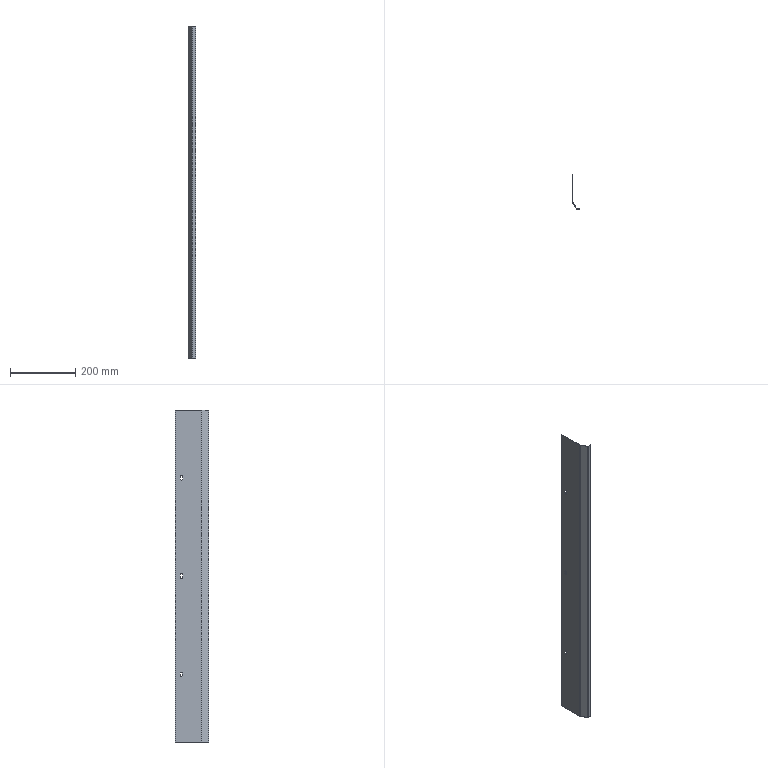Part | 1 solid | 37 faces | box 23.5 x 102.651 x 1015 mm | volume 117216 mm3 | plane 24 | cylinder 13 | commonest cylinder face diameters 7 x6 6 x3 1 x2 3 x2
STEP:
#1=CARTESIAN_POINT('',(0.,-16.,-296.5));
#2=VERTEX_POINT('',#1);
#3=CARTESIAN_POINT('',(0.,-19.,-293.5));
#4=VERTEX_POINT('',#3);
#5=CARTESIAN_POINT('',(0.,-19.,-296.5));
#6=DIRECTION('',(1.,0.,0.));
#7=DIRECTION('',(0.,1.,0.));
#8=AXIS2_PLACEMENT_3D('',#5,#6,#7);
#9=CIRCLE('',#8,3.);
#10=EDGE_CURVE('',#2,#4,#9,.T.);
#11=ORIENTED_EDGE('',*,*,#10,.T.);
#12=CARTESIAN_POINT('',(-1.,-19.,-293.5));
#13=VERTEX_POINT('',#12);
#14=CARTESIAN_POINT('',(9.,-19.,-293.5));
#15=DIRECTION('',(-1.,0.,0.));
#16=VECTOR('',#15,1000.);
#17=LINE('',#14,#16);
#18=EDGE_CURVE('',#4,#13,#17,.T.);
#19=ORIENTED_EDGE('',*,*,#18,.T.);
#20=CARTESIAN_POINT('',(-1.,-16.,-296.5));
#21=VERTEX_POINT('',#20);
#22=CARTESIAN_POINT('',(-1.,-19.,-296.5));
#23=DIRECTION('',(-1.,0.,0.));
#24=DIRECTION('',(0.,0.,1.));
#25=AXIS2_PLACEMENT_3D('',#22,#23,#24);
#26=CIRCLE('',#25,3.);
#27=EDGE_CURVE('',#13,#21,#26,.T.);
#28=ORIENTED_EDGE('',*,*,#27,.T.);
#29=CARTESIAN_POINT('',(9.,-16.,-296.5));
#30=DIRECTION('',(-1.,0.,0.));
#31=VECTOR('',#30,1000.);
#32=LINE('',#29,#31);
#33=EDGE_CURVE('',#2,#21,#32,.T.);
#34=ORIENTED_EDGE('',*,*,#33,.F.);
#35=EDGE_LOOP('',(#11,#19,#28,#34));
#36=FACE_OUTER_BOUND('',#35,.T.);
#37=CARTESIAN_POINT('',(9.,-19.,-296.5));
#38=DIRECTION('',(-1.,0.,0.));
#39=DIRECTION('',(0.,0.,1.));
#40=AXIS2_PLACEMENT_3D('',#37,#38,#39);
#41=CYLINDRICAL_SURFACE('',#40,3.);
#42=ADVANCED_FACE('',(#36),#41,.F.);
#43=CARTESIAN_POINT('',(0.,-15.5,303.5));
#44=VERTEX_POINT('',#43);
#45=CARTESIAN_POINT('',(0.,-19.,307.));
#46=VERTEX_POINT('',#45);
#47=CARTESIAN_POINT('',(0.,-19.,303.5));
#48=DIRECTION('',(1.,0.,0.));
#49=DIRECTION('',(0.,1.,0.));
#50=AXIS2_PLACEMENT_3D('',#47,#48,#49);
#51=CIRCLE('',#50,3.5);
#52=EDGE_CURVE('',#44,#46,#51,.T.);
#53=ORIENTED_EDGE('',*,*,#52,.T.);
#54=CARTESIAN_POINT('',(-1.,-19.,307.));
#55=VERTEX_POINT('',#54);
#56=CARTESIAN_POINT('',(9.,-19.,307.));
#57=DIRECTION('',(-1.,0.,0.));
#58=VECTOR('',#57,1000.);
#59=LINE('',#56,#58);
#60=EDGE_CURVE('',#46,#55,#59,.T.);
#61=ORIENTED_EDGE('',*,*,#60,.T.);
#62=CARTESIAN_POINT('',(-1.,-15.5,303.5));
#63=VERTEX_POINT('',#62);
#64=CARTESIAN_POINT('',(-1.,-19.,303.5));
#65=DIRECTION('',(-1.,0.,0.));
#66=DIRECTION('',(0.,0.,1.));
#67=AXIS2_PLACEMENT_3D('',#64,#65,#66);
#68=CIRCLE('',#67,3.5);
#69=EDGE_CURVE('',#55,#63,#68,.T.);
#70=ORIENTED_EDGE('',*,*,#69,.T.);
#71=CARTESIAN_POINT('',(9.,-15.5,303.5));
#72=DIRECTION('',(-1.,0.,0.));
#73=VECTOR('',#72,1000.);
#74=LINE('',#71,#73);
#75=EDGE_CURVE('',#44,#63,#74,.T.);
#76=ORIENTED_EDGE('',*,*,#75,.F.);
#77=EDGE_LOOP('',(#53,#61,#70,#76));
#78=FACE_OUTER_BOUND('',#77,.T.);
#79=CARTESIAN_POINT('',(9.,-19.,303.5));
#80=DIRECTION('',(-1.,0.,0.));
#81=DIRECTION('',(0.,0.,1.));
#82=AXIS2_PLACEMENT_3D('',#79,#80,#81);
#83=CYLINDRICAL_SURFACE('',#82,3.5);
#84=ADVANCED_FACE('',(#78),#83,.F.);
#85=CARTESIAN_POINT('',(0.,-15.5,3.5));
#86=VERTEX_POINT('',#85);
#87=CARTESIAN_POINT('',(0.,-19.,7.));
#88=VERTEX_POINT('',#87);
#89=CARTESIAN_POINT('',(0.,-19.,3.5));
#90=DIRECTION('',(1.,0.,0.));
#91=DIRECTION('',(0.,1.,0.));
#92=AXIS2_PLACEMENT_3D('',#89,#90,#91);
#93=CIRCLE('',#92,3.5);
#94=EDGE_CURVE('',#86,#88,#93,.T.);
#95=ORIENTED_EDGE('',*,*,#94,.T.);
#96=CARTESIAN_POINT('',(-1.,-19.,7.));
#97=VERTEX_POINT('',#96);
#98=CARTESIAN_POINT('',(9.,-19.,7.));
#99=DIRECTION('',(-1.,0.,0.));
#100=VECTOR('',#99,1000.);
#101=LINE('',#98,#100);
#102=EDGE_CURVE('',#88,#97,#101,.T.);
#103=ORIENTED_EDGE('',*,*,#102,.T.);
#104=CARTESIAN_POINT('',(-1.,-15.5,3.5));
#105=VERTEX_POINT('',#104);
#106=CARTESIAN_POINT('',(-1.,-19.,3.5));
#107=DIRECTION('',(-1.,0.,0.));
#108=DIRECTION('',(0.,0.,1.));
#109=AXIS2_PLACEMENT_3D('',#106,#107,#108);
#110=CIRCLE('',#109,3.5);
#111=EDGE_CURVE('',#97,#105,#110,.T.);
#112=ORIENTED_EDGE('',*,*,#111,.T.);
#113=CARTESIAN_POINT('',(9.,-15.5,3.5));
#114=DIRECTION('',(-1.,0.,0.));
#115=VECTOR('',#114,1000.);
#116=LINE('',#113,#115);
#117=EDGE_CURVE('',#86,#105,#116,.T.);
#118=ORIENTED_EDGE('',*,*,#117,.F.);
#119=EDGE_LOOP('',(#95,#103,#112,#118));
#120=FACE_OUTER_BOUND('',#119,.T.);
#121=CARTESIAN_POINT('',(9.,-19.,3.5));
#122=DIRECTION('',(-1.,0.,0.));
#123=DIRECTION('',(0.,0.,1.));
#124=AXIS2_PLACEMENT_3D('',#121,#122,#123);
#125=CYLINDRICAL_SURFACE('',#124,3.5);
#126=ADVANCED_FACE('',(#120),#125,.F.);
#127=CARTESIAN_POINT('',(0.06699,-80.116,507.5));
#128=VERTEX_POINT('',#127);
#129=CARTESIAN_POINT('',(-0.799,-80.616,507.5));
#130=VERTEX_POINT('',#129);
#131=CARTESIAN_POINT('',(0.06699,-80.116,507.5));
#132=DIRECTION('',(-0.866,-0.5,0.));
#133=VECTOR('',#132,1000.);
#134=LINE('',#131,#133);
#135=EDGE_CURVE('',#128,#130,#134,.T.);
#136=ORIENTED_EDGE('',*,*,#135,.F.);
#137=CARTESIAN_POINT('',(0.,-79.866,507.5));
#138=VERTEX_POINT('',#137);
#139=CARTESIAN_POINT('',(0.5,-79.866,507.5));
#140=DIRECTION('',(0.,0.,1.));
#141=DIRECTION('',(-1.,0.,0.));
#142=AXIS2_PLACEMENT_3D('',#139,#140,#141);
#143=CIRCLE('',#142,0.5);
#144=EDGE_CURVE('',#138,#128,#143,.T.);
#145=ORIENTED_EDGE('',*,*,#144,.F.);
#146=CARTESIAN_POINT('',(-1.,-79.866,507.5));
#147=VERTEX_POINT('',#146);
#148=CARTESIAN_POINT('',(-1.,-79.866,507.5));
#149=DIRECTION('',(1.,0.,0.));
#150=VECTOR('',#149,1000.);
#151=LINE('',#148,#150);
#152=EDGE_CURVE('',#147,#138,#151,.T.);
#153=ORIENTED_EDGE('',*,*,#152,.F.);
#154=CARTESIAN_POINT('',(0.5,-79.866,507.5));
#155=DIRECTION('',(0.,0.,1.));
#156=DIRECTION('',(1.,0.,0.));
#157=AXIS2_PLACEMENT_3D('',#154,#155,#156);
#158=CIRCLE('',#157,1.5);
#159=EDGE_CURVE('',#147,#130,#158,.T.);
#160=ORIENTED_EDGE('',*,*,#159,.T.);
#161=EDGE_LOOP('',(#136,#145,#153,#160));
#162=FACE_OUTER_BOUND('',#161,.T.);
#163=CARTESIAN_POINT('',(0.06699,-80.116,507.5));
#164=DIRECTION('',(0.,0.,1.));
#165=DIRECTION('',(1.,0.,0.));
#166=AXIS2_PLACEMENT_3D('',#163,#164,#165);
#167=PLANE('',#166);
#168=ADVANCED_FACE('',(#162),#167,.T.);
#169=CARTESIAN_POINT('',(12.356,-101.401,507.5));
#170=VERTEX_POINT('',#169);
#171=CARTESIAN_POINT('',(0.,-80.,507.5));
#172=DIRECTION('',(0.5,-0.866,0.));
#173=VECTOR('',#172,1000.);
#174=LINE('',#171,#173);
#175=EDGE_CURVE('',#128,#170,#174,.T.);
#176=ORIENTED_EDGE('',*,*,#175,.F.);
#177=ORIENTED_EDGE('',*,*,#135,.T.);
#178=CARTESIAN_POINT('',(11.49,-101.901,507.5));
#179=VERTEX_POINT('',#178);
#180=CARTESIAN_POINT('',(-0.866,-80.5,507.5));
#181=DIRECTION('',(0.5,-0.866,0.));
#182=VECTOR('',#181,1000.);
#183=LINE('',#180,#182);
#184=EDGE_CURVE('',#130,#179,#183,.T.);
#185=ORIENTED_EDGE('',*,*,#184,.T.);
#186=CARTESIAN_POINT('',(11.49,-101.901,507.5));
#187=DIRECTION('',(0.866,0.5,0.));
#188=VECTOR('',#187,1000.);
#189=LINE('',#186,#188);
#190=EDGE_CURVE('',#179,#170,#189,.T.);
#191=ORIENTED_EDGE('',*,*,#190,.T.);
#192=EDGE_LOOP('',(#176,#177,#185,#191));
#193=FACE_OUTER_BOUND('',#192,.T.);
#194=CARTESIAN_POINT('',(-1.,-79.866,507.5));
#195=DIRECTION('',(0.,0.,1.));
#196=DIRECTION('',(1.,0.,0.));
#197=AXIS2_PLACEMENT_3D('',#194,#195,#196);
#198=PLANE('',#197);
#199=ADVANCED_FACE('',(#193),#198,.T.);
#200=CARTESIAN_POINT('',(0.,-79.866,-507.5));
#201=VERTEX_POINT('',#200);
#202=CARTESIAN_POINT('',(-1.,-79.866,-507.5));
#203=VERTEX_POINT('',#202);
#204=CARTESIAN_POINT('',(0.,-79.866,-507.5));
#205=DIRECTION('',(-1.,0.,0.));
#206=VECTOR('',#205,1000.);
#207=LINE('',#204,#206);
#208=EDGE_CURVE('',#201,#203,#207,.T.);
#209=ORIENTED_EDGE('',*,*,#208,.F.);
#210=CARTESIAN_POINT('',(0.06699,-80.116,-507.5));
#211=VERTEX_POINT('',#210);
#212=CARTESIAN_POINT('',(0.5,-79.866,-507.5));
#213=DIRECTION('',(0.,0.,1.));
#214=DIRECTION('',(-1.,0.,0.));
#215=AXIS2_PLACEMENT_3D('',#212,#213,#214);
#216=CIRCLE('',#215,0.5);
#217=EDGE_CURVE('',#201,#211,#216,.T.);
#218=ORIENTED_EDGE('',*,*,#217,.T.);
#219=CARTESIAN_POINT('',(-0.799,-80.616,-507.5));
#220=VERTEX_POINT('',#219);
#221=CARTESIAN_POINT('',(-0.799,-80.616,-507.5));
#222=DIRECTION('',(0.866,0.5,0.));
#223=VECTOR('',#222,1000.);
#224=LINE('',#221,#223);
#225=EDGE_CURVE('',#220,#211,#224,.T.);
#226=ORIENTED_EDGE('',*,*,#225,.F.);
#227=CARTESIAN_POINT('',(0.5,-79.866,-507.5));
#228=DIRECTION('',(0.,0.,1.));
#229=DIRECTION('',(1.,0.,0.));
#230=AXIS2_PLACEMENT_3D('',#227,#228,#229);
#231=CIRCLE('',#230,1.5);
#232=EDGE_CURVE('',#203,#220,#231,.T.);
#233=ORIENTED_EDGE('',*,*,#232,.F.);
#234=EDGE_LOOP('',(#209,#218,#226,#233));
#235=FACE_OUTER_BOUND('',#234,.T.);
#236=CARTESIAN_POINT('',(0.,-79.866,-507.5));
#237=DIRECTION('',(0.,0.,-1.));
#238=DIRECTION('',(-1.,0.,0.));
#239=AXIS2_PLACEMENT_3D('',#236,#237,#238);
#240=PLANE('',#239);
#241=ADVANCED_FACE('',(#235),#240,.T.);
#242=CARTESIAN_POINT('',(0.,0.,-507.5));
#243=VERTEX_POINT('',#242);
#244=CARTESIAN_POINT('',(0.,0.,-507.5));
#245=DIRECTION('',(0.,-1.,0.));
#246=VECTOR('',#245,1000.);
#247=LINE('',#244,#246);
#248=EDGE_CURVE('',#243,#201,#247,.T.);
#249=ORIENTED_EDGE('',*,*,#248,.T.);
#250=ORIENTED_EDGE('',*,*,#208,.T.);
#251=CARTESIAN_POINT('',(-1.,0.,-507.5));
#252=VERTEX_POINT('',#251);
#253=CARTESIAN_POINT('',(-1.,0.,-507.5));
#254=DIRECTION('',(0.,-1.,0.));
#255=VECTOR('',#254,1000.);
#256=LINE('',#253,#255);
#257=EDGE_CURVE('',#252,#203,#256,.T.);
#258=ORIENTED_EDGE('',*,*,#257,.F.);
#259=CARTESIAN_POINT('',(-1.,0.,-507.5));
#260=DIRECTION('',(1.,0.,0.));
#261=VECTOR('',#260,1000.);
#262=LINE('',#259,#261);
#263=EDGE_CURVE('',#252,#243,#262,.T.);
#264=ORIENTED_EDGE('',*,*,#263,.T.);
#265=EDGE_LOOP('',(#249,#250,#258,#264));
#266=FACE_OUTER_BOUND('',#265,.T.);
#267=CARTESIAN_POINT('',(-0.799,-80.616,-507.5));
#268=DIRECTION('',(0.,0.,-1.));
#269=DIRECTION('',(-1.,0.,0.));
#270=AXIS2_PLACEMENT_3D('',#267,#268,#269);
#271=PLANE('',#270);
#272=ADVANCED_FACE('',(#266),#271,.T.);
#273=CARTESIAN_POINT('',(12.789,-101.651,507.5));
#274=VERTEX_POINT('',#273);
#275=CARTESIAN_POINT('',(12.789,-102.651,507.5));
#276=VERTEX_POINT('',#275);
#277=CARTESIAN_POINT('',(12.789,-101.651,507.5));
#278=DIRECTION('',(0.,-1.,0.));
#279=VECTOR('',#278,1000.);
#280=LINE('',#277,#279);
#281=EDGE_CURVE('',#274,#276,#280,.T.);
#282=ORIENTED_EDGE('',*,*,#281,.F.);
#283=CARTESIAN_POINT('',(12.789,-101.151,507.5));
#284=DIRECTION('',(0.,0.,1.));
#285=DIRECTION('',(-1.,0.,0.));
#286=AXIS2_PLACEMENT_3D('',#283,#284,#285);
#287=CIRCLE('',#286,0.5);
#288=EDGE_CURVE('',#170,#274,#287,.T.);
#289=ORIENTED_EDGE('',*,*,#288,.F.);
#290=ORIENTED_EDGE('',*,*,#190,.F.);
#291=CARTESIAN_POINT('',(12.789,-101.151,507.5));
#292=DIRECTION('',(0.,0.,1.));
#293=DIRECTION('',(1.,0.,0.));
#294=AXIS2_PLACEMENT_3D('',#291,#292,#293);
#295=CIRCLE('',#294,1.5);
#296=EDGE_CURVE('',#179,#276,#295,.T.);
#297=ORIENTED_EDGE('',*,*,#296,.T.);
#298=EDGE_LOOP('',(#282,#289,#290,#297));
#299=FACE_OUTER_BOUND('',#298,.T.);
#300=CARTESIAN_POINT('',(12.789,-101.651,507.5));
#301=DIRECTION('',(0.,0.,1.));
#302=DIRECTION('',(1.,0.,0.));
#303=AXIS2_PLACEMENT_3D('',#300,#301,#302);
#304=PLANE('',#303);
#305=ADVANCED_FACE('',(#299),#304,.T.);
#306=CARTESIAN_POINT('',(22.5,-101.651,507.5));
#307=VERTEX_POINT('',#306);
#308=CARTESIAN_POINT('',(12.5,-101.651,507.5));
#309=DIRECTION('',(1.,0.,0.));
#310=VECTOR('',#309,1000.);
#311=LINE('',#308,#310);
#312=EDGE_CURVE('',#274,#307,#311,.T.);
#313=ORIENTED_EDGE('',*,*,#312,.F.);
#314=ORIENTED_EDGE('',*,*,#281,.T.);
#315=CARTESIAN_POINT('',(22.5,-102.651,507.5));
#316=VERTEX_POINT('',#315);
#317=CARTESIAN_POINT('',(12.5,-102.651,507.5));
#318=DIRECTION('',(1.,0.,0.));
#319=VECTOR('',#318,1000.);
#320=LINE('',#317,#319);
#321=EDGE_CURVE('',#276,#316,#320,.T.);
#322=ORIENTED_EDGE('',*,*,#321,.T.);
#323=CARTESIAN_POINT('',(22.5,-101.651,507.5));
#324=DIRECTION('',(0.,-1.,0.));
#325=VECTOR('',#324,1000.);
#326=LINE('',#323,#325);
#327=EDGE_CURVE('',#307,#316,#326,.T.);
#328=ORIENTED_EDGE('',*,*,#327,.F.);
#329=EDGE_LOOP('',(#313,#314,#322,#328));
#330=FACE_OUTER_BOUND('',#329,.T.);
#331=CARTESIAN_POINT('',(11.49,-101.901,507.5));
#332=DIRECTION('',(0.,0.,1.));
#333=DIRECTION('',(1.,0.,0.));
#334=AXIS2_PLACEMENT_3D('',#331,#332,#333);
#335=PLANE('',#334);
#336=ADVANCED_FACE('',(#330),#335,.T.);
#337=CARTESIAN_POINT('',(12.356,-101.401,-507.5));
#338=VERTEX_POINT('',#337);
#339=CARTESIAN_POINT('',(11.49,-101.901,-507.5));
#340=VERTEX_POINT('',#339);
#341=CARTESIAN_POINT('',(12.356,-101.401,-507.5));
#342=DIRECTION('',(-0.866,-0.5,0.));
#343=VECTOR('',#342,1000.);
#344=LINE('',#341,#343);
#345=EDGE_CURVE('',#338,#340,#344,.T.);
#346=ORIENTED_EDGE('',*,*,#345,.F.);
#347=CARTESIAN_POINT('',(12.789,-101.651,-507.5));
#348=VERTEX_POINT('',#347);
#349=CARTESIAN_POINT('',(12.789,-101.151,-507.5));
#350=DIRECTION('',(0.,0.,1.));
#351=DIRECTION('',(-1.,0.,0.));
#352=AXIS2_PLACEMENT_3D('',#349,#350,#351);
#353=CIRCLE('',#352,0.5);
#354=EDGE_CURVE('',#338,#348,#353,.T.);
#355=ORIENTED_EDGE('',*,*,#354,.T.);
#356=CARTESIAN_POINT('',(12.789,-102.651,-507.5));
#357=VERTEX_POINT('',#356);
#358=CARTESIAN_POINT('',(12.789,-102.651,-507.5));
#359=DIRECTION('',(0.,1.,0.));
#360=VECTOR('',#359,1000.);
#361=LINE('',#358,#360);
#362=EDGE_CURVE('',#357,#348,#361,.T.);
#363=ORIENTED_EDGE('',*,*,#362,.F.);
#364=CARTESIAN_POINT('',(12.789,-101.151,-507.5));
#365=DIRECTION('',(0.,0.,1.));
#366=DIRECTION('',(1.,0.,0.));
#367=AXIS2_PLACEMENT_3D('',#364,#365,#366);
#368=CIRCLE('',#367,1.5);
#369=EDGE_CURVE('',#340,#357,#368,.T.);
#370=ORIENTED_EDGE('',*,*,#369,.F.);
#371=EDGE_LOOP('',(#346,#355,#363,#370));
#372=FACE_OUTER_BOUND('',#371,.T.);
#373=CARTESIAN_POINT('',(12.356,-101.401,-507.5));
#374=DIRECTION('',(0.,0.,-1.));
#375=DIRECTION('',(-1.,0.,0.));
#376=AXIS2_PLACEMENT_3D('',#373,#374,#375);
#377=PLANE('',#376);
#378=ADVANCED_FACE('',(#372),#377,.T.);
#379=CARTESIAN_POINT('',(0.,-80.,-507.5));
#380=DIRECTION('',(0.5,-0.866,0.));
#381=VECTOR('',#380,1000.);
#382=LINE('',#379,#381);
#383=EDGE_CURVE('',#211,#338,#382,.T.);
#384=ORIENTED_EDGE('',*,*,#383,.T.);
#385=ORIENTED_EDGE('',*,*,#345,.T.);
#386=CARTESIAN_POINT('',(-0.866,-80.5,-507.5));
#387=DIRECTION('',(0.5,-0.866,0.));
#388=VECTOR('',#387,1000.);
#389=LINE('',#386,#388);
#390=EDGE_CURVE('',#220,#340,#389,.T.);
#391=ORIENTED_EDGE('',*,*,#390,.F.);
#392=ORIENTED_EDGE('',*,*,#225,.T.);
#393=EDGE_LOOP('',(#384,#385,#391,#392));
#394=FACE_OUTER_BOUND('',#393,.T.);
#395=CARTESIAN_POINT('',(12.789,-102.651,-507.5));
#396=DIRECTION('',(0.,0.,-1.));
#397=DIRECTION('',(-1.,0.,0.));
#398=AXIS2_PLACEMENT_3D('',#395,#396,#397);
#399=PLANE('',#398);
#400=ADVANCED_FACE('',(#394),#399,.T.);
#401=CARTESIAN_POINT('',(22.5,-102.651,-507.5));
#402=VERTEX_POINT('',#401);
#403=CARTESIAN_POINT('',(12.5,-102.651,-507.5));
#404=DIRECTION('',(1.,0.,0.));
#405=VECTOR('',#404,1000.);
#406=LINE('',#403,#405);
#407=EDGE_CURVE('',#357,#402,#406,.T.);
#408=ORIENTED_EDGE('',*,*,#407,.T.);
#409=CARTESIAN_POINT('',(22.5,-102.651,507.5));
#410=DIRECTION('',(0.,0.,-1.));
#411=VECTOR('',#410,1000.);
#412=LINE('',#409,#411);
#413=EDGE_CURVE('',#316,#402,#412,.T.);
#414=ORIENTED_EDGE('',*,*,#413,.F.);
#415=ORIENTED_EDGE('',*,*,#321,.F.);
#416=CARTESIAN_POINT('',(12.789,-102.651,507.5));
#417=DIRECTION('',(0.,0.,-1.));
#418=VECTOR('',#417,1000.);
#419=LINE('',#416,#418);
#420=EDGE_CURVE('',#276,#357,#419,.T.);
#421=ORIENTED_EDGE('',*,*,#420,.T.);
#422=EDGE_LOOP('',(#408,#414,#415,#421));
#423=FACE_OUTER_BOUND('',#422,.T.);
#424=CARTESIAN_POINT('',(12.5,-102.651,507.5));
#425=DIRECTION('',(0.,1.,0.));
#426=DIRECTION('',(0.,0.,1.));
#427=AXIS2_PLACEMENT_3D('',#424,#425,#426);
#428=PLANE('',#427);
#429=ADVANCED_FACE('',(#423),#428,.F.);
#430=CARTESIAN_POINT('',(22.5,-101.651,-507.5));
#431=VERTEX_POINT('',#430);
#432=CARTESIAN_POINT('',(22.5,-101.651,-507.5));
#433=DIRECTION('',(0.,-1.,0.));
#434=VECTOR('',#433,1000.);
#435=LINE('',#432,#434);
#436=EDGE_CURVE('',#431,#402,#435,.T.);
#437=ORIENTED_EDGE('',*,*,#436,.F.);
#438=CARTESIAN_POINT('',(22.5,-101.651,507.5));
#439=DIRECTION('',(0.,0.,-1.));
#440=VECTOR('',#439,1000.);
#441=LINE('',#438,#440);
#442=EDGE_CURVE('',#307,#431,#441,.T.);
#443=ORIENTED_EDGE('',*,*,#442,.F.);
#444=ORIENTED_EDGE('',*,*,#327,.T.);
#445=ORIENTED_EDGE('',*,*,#413,.T.);
#446=EDGE_LOOP('',(#437,#443,#444,#445));
#447=FACE_OUTER_BOUND('',#446,.T.);
#448=CARTESIAN_POINT('',(22.5,-101.651,507.5));
#449=DIRECTION('',(1.,0.,0.));
#450=DIRECTION('',(0.,0.,-1.));
#451=AXIS2_PLACEMENT_3D('',#448,#449,#450);
#452=PLANE('',#451);
#453=ADVANCED_FACE('',(#447),#452,.T.);
#454=CARTESIAN_POINT('',(12.5,-101.651,-507.5));
#455=DIRECTION('',(1.,0.,0.));
#456=VECTOR('',#455,1000.);
#457=LINE('',#454,#456);
#458=EDGE_CURVE('',#348,#431,#457,.T.);
#459=ORIENTED_EDGE('',*,*,#458,.F.);
#460=CARTESIAN_POINT('',(12.789,-101.651,507.5));
#461=DIRECTION('',(0.,0.,-1.));
#462=VECTOR('',#461,1000.);
#463=LINE('',#460,#462);
#464=EDGE_CURVE('',#274,#348,#463,.T.);
#465=ORIENTED_EDGE('',*,*,#464,.F.);
#466=ORIENTED_EDGE('',*,*,#312,.T.);
#467=ORIENTED_EDGE('',*,*,#442,.T.);
#468=EDGE_LOOP('',(#459,#465,#466,#467));
#469=FACE_OUTER_BOUND('',#468,.T.);
#470=CARTESIAN_POINT('',(12.5,-101.651,507.5));
#471=DIRECTION('',(0.,1.,0.));
#472=DIRECTION('',(0.,0.,1.));
#473=AXIS2_PLACEMENT_3D('',#470,#471,#472);
#474=PLANE('',#473);
#475=ADVANCED_FACE('',(#469),#474,.T.);
#476=ORIENTED_EDGE('',*,*,#354,.F.);
#477=CARTESIAN_POINT('',(12.356,-101.401,507.5));
#478=DIRECTION('',(0.,0.,-1.));
#479=VECTOR('',#478,1000.);
#480=LINE('',#477,#479);
#481=EDGE_CURVE('',#170,#338,#480,.T.);
#482=ORIENTED_EDGE('',*,*,#481,.F.);
#483=ORIENTED_EDGE('',*,*,#288,.T.);
#484=ORIENTED_EDGE('',*,*,#464,.T.);
#485=EDGE_LOOP('',(#476,#482,#483,#484));
#486=FACE_OUTER_BOUND('',#485,.T.);
#487=CARTESIAN_POINT('',(12.789,-101.151,507.5));
#488=DIRECTION('',(0.,0.,-1.));
#489=DIRECTION('',(-1.,0.,0.));
#490=AXIS2_PLACEMENT_3D('',#487,#488,#489);
#491=CYLINDRICAL_SURFACE('',#490,0.5);
#492=ADVANCED_FACE('',(#486),#491,.F.);
#493=ORIENTED_EDGE('',*,*,#383,.F.);
#494=CARTESIAN_POINT('',(0.06699,-80.116,507.5));
#495=DIRECTION('',(0.,0.,-1.));
#496=VECTOR('',#495,1000.);
#497=LINE('',#494,#496);
#498=EDGE_CURVE('',#128,#211,#497,.T.);
#499=ORIENTED_EDGE('',*,*,#498,.F.);
#500=ORIENTED_EDGE('',*,*,#175,.T.);
#501=ORIENTED_EDGE('',*,*,#481,.T.);
#502=EDGE_LOOP('',(#493,#499,#500,#501));
#503=FACE_OUTER_BOUND('',#502,.T.);
#504=CARTESIAN_POINT('',(0.,-80.,507.5));
#505=DIRECTION('',(0.866,0.5,0.));
#506=DIRECTION('',(-0.5,0.866,0.));
#507=AXIS2_PLACEMENT_3D('',#504,#505,#506);
#508=PLANE('',#507);
#509=ADVANCED_FACE('',(#503),#508,.T.);
#510=ORIENTED_EDGE('',*,*,#217,.F.);
#511=CARTESIAN_POINT('',(0.,-79.866,507.5));
#512=DIRECTION('',(0.,0.,-1.));
#513=VECTOR('',#512,1000.);
#514=LINE('',#511,#513);
#515=EDGE_CURVE('',#138,#201,#514,.T.);
#516=ORIENTED_EDGE('',*,*,#515,.F.);
#517=ORIENTED_EDGE('',*,*,#144,.T.);
#518=ORIENTED_EDGE('',*,*,#498,.T.);
#519=EDGE_LOOP('',(#510,#516,#517,#518));
#520=FACE_OUTER_BOUND('',#519,.T.);
#521=CARTESIAN_POINT('',(0.5,-79.866,507.5));
#522=DIRECTION('',(0.,0.,-1.));
#523=DIRECTION('',(-1.,0.,0.));
#524=AXIS2_PLACEMENT_3D('',#521,#522,#523);
#525=CYLINDRICAL_SURFACE('',#524,0.5);
#526=ADVANCED_FACE('',(#520),#525,.F.);
#527=CARTESIAN_POINT('',(0.,-22.,-303.5));
#528=VERTEX_POINT('',#527);
#529=CARTESIAN_POINT('',(0.,-16.,-303.5));
#530=VERTEX_POINT('',#529);
#531=CARTESIAN_POINT('',(0.,-19.,-303.5));
#532=DIRECTION('',(1.,0.,0.));
#533=DIRECTION('',(0.,1.,0.));
#534=AXIS2_PLACEMENT_3D('',#531,#532,#533);
#535=CIRCLE('',#534,3.);
#536=EDGE_CURVE('',#528,#530,#535,.T.);
#537=ORIENTED_EDGE('',*,*,#536,.F.);
#538=CARTESIAN_POINT('',(0.,-22.,-296.5));
#539=VERTEX_POINT('',#538);
#540=CARTESIAN_POINT('',(0.,-22.,507.5));
#541=DIRECTION('',(0.,0.,-1.));
#542=VECTOR('',#541,1000.);
#543=LINE('',#540,#542);
#544=EDGE_CURVE('',#539,#528,#543,.T.);
#545=ORIENTED_EDGE('',*,*,#544,.F.);
#546=CARTESIAN_POINT('',(0.,-19.,-296.5));
#547=DIRECTION('',(1.,0.,0.));
#548=DIRECTION('',(0.,1.,0.));
#549=AXIS2_PLACEMENT_3D('',#546,#547,#548);
#550=CIRCLE('',#549,3.);
#551=EDGE_CURVE('',#4,#539,#550,.T.);
#552=ORIENTED_EDGE('',*,*,#551,.F.);
#553=ORIENTED_EDGE('',*,*,#10,.F.);
#554=CARTESIAN_POINT('',(0.,-16.,507.5));
#555=DIRECTION('',(0.,0.,1.));
#556=VECTOR('',#555,1000.);
#557=LINE('',#554,#556);
#558=EDGE_CURVE('',#530,#2,#557,.T.);
#559=ORIENTED_EDGE('',*,*,#558,.F.);
#560=EDGE_LOOP('',(#537,#545,#552,#553,#559));
#561=FACE_BOUND('',#560,.T.);
#562=CARTESIAN_POINT('',(0.,-22.5,296.5));
#563=VERTEX_POINT('',#562);
#564=CARTESIAN_POINT('',(0.,-15.5,296.5));
#565=VERTEX_POINT('',#564);
#566=CARTESIAN_POINT('',(0.,-19.,296.5));
#567=DIRECTION('',(1.,0.,0.));
#568=DIRECTION('',(0.,1.,0.));
#569=AXIS2_PLACEMENT_3D('',#566,#567,#568);
#570=CIRCLE('',#569,3.5);
#571=EDGE_CURVE('',#563,#565,#570,.T.);
#572=ORIENTED_EDGE('',*,*,#571,.F.);
#573=CARTESIAN_POINT('',(0.,-22.5,303.5));
#574=VERTEX_POINT('',#573);
#575=CARTESIAN_POINT('',(0.,-22.5,507.5));
#576=DIRECTION('',(0.,0.,-1.));
#577=VECTOR('',#576,1000.);
#578=LINE('',#575,#577);
#579=EDGE_CURVE('',#574,#563,#578,.T.);
#580=ORIENTED_EDGE('',*,*,#579,.F.);
#581=CARTESIAN_POINT('',(0.,-19.,303.5));
#582=DIRECTION('',(1.,0.,0.));
#583=DIRECTION('',(0.,1.,0.));
#584=AXIS2_PLACEMENT_3D('',#581,#582,#583);
#585=CIRCLE('',#584,3.5);
#586=EDGE_CURVE('',#46,#574,#585,.T.);
#587=ORIENTED_EDGE('',*,*,#586,.F.);
#588=ORIENTED_EDGE('',*,*,#52,.F.);
#589=CARTESIAN_POINT('',(0.,-15.5,507.5));
#590=DIRECTION('',(0.,0.,1.));
#591=VECTOR('',#590,1000.);
#592=LINE('',#589,#591);
#593=EDGE_CURVE('',#565,#44,#592,.T.);
#594=ORIENTED_EDGE('',*,*,#593,.F.);
#595=EDGE_LOOP('',(#572,#580,#587,#588,#594));
#596=FACE_BOUND('',#595,.T.);
#597=CARTESIAN_POINT('',(0.,-22.5,-3.5));
#598=VERTEX_POINT('',#597);
#599=CARTESIAN_POINT('',(0.,-15.5,-3.5));
#600=VERTEX_POINT('',#599);
#601=CARTESIAN_POINT('',(0.,-19.,-3.5));
#602=DIRECTION('',(1.,0.,0.));
#603=DIRECTION('',(0.,1.,0.));
#604=AXIS2_PLACEMENT_3D('',#601,#602,#603);
#605=CIRCLE('',#604,3.5);
#606=EDGE_CURVE('',#598,#600,#605,.T.);
#607=ORIENTED_EDGE('',*,*,#606,.F.);
#608=CARTESIAN_POINT('',(0.,-22.5,3.5));
#609=VERTEX_POINT('',#608);
#610=CARTESIAN_POINT('',(0.,-22.5,507.5));
#611=DIRECTION('',(0.,0.,-1.));
#612=VECTOR('',#611,1000.);
#613=LINE('',#610,#612);
#614=EDGE_CURVE('',#609,#598,#613,.T.);
#615=ORIENTED_EDGE('',*,*,#614,.F.);
#616=CARTESIAN_POINT('',(0.,-19.,3.5));
#617=DIRECTION('',(1.,0.,0.));
#618=DIRECTION('',(0.,1.,0.));
#619=AXIS2_PLACEMENT_3D('',#616,#617,#618);
#620=CIRCLE('',#619,3.5);
#621=EDGE_CURVE('',#88,#609,#620,.T.);
#622=ORIENTED_EDGE('',*,*,#621,.F.);
#623=ORIENTED_EDGE('',*,*,#94,.F.);
#624=CARTESIAN_POINT('',(0.,-15.5,507.5));
#625=DIRECTION('',(0.,0.,1.));
#626=VECTOR('',#625,1000.);
#627=LINE('',#624,#626);
#628=EDGE_CURVE('',#600,#86,#627,.T.);
#629=ORIENTED_EDGE('',*,*,#628,.F.);
#630=EDGE_LOOP('',(#607,#615,#622,#623,#629));
#631=FACE_BOUND('',#630,.T.);
#632=ORIENTED_EDGE('',*,*,#248,.F.);
#633=CARTESIAN_POINT('',(0.,0.,507.5));
#634=VERTEX_POINT('',#633);
#635=CARTESIAN_POINT('',(0.,0.,507.5));
#636=DIRECTION('',(0.,0.,-1.));
#637=VECTOR('',#636,1000.);
#638=LINE('',#635,#637);
#639=EDGE_CURVE('',#634,#243,#638,.T.);
#640=ORIENTED_EDGE('',*,*,#639,.F.);
#641=CARTESIAN_POINT('',(0.,0.,507.5));
#642=DIRECTION('',(0.,-1.,0.));
#643=VECTOR('',#642,1000.);
#644=LINE('',#641,#643);
#645=EDGE_CURVE('',#634,#138,#644,.T.);
#646=ORIENTED_EDGE('',*,*,#645,.T.);
#647=ORIENTED_EDGE('',*,*,#515,.T.);
#648=EDGE_LOOP('',(#632,#640,#646,#647));
#649=FACE_OUTER_BOUND('',#648,.T.);
#650=CARTESIAN_POINT('',(0.,0.,507.5));
#651=DIRECTION('',(1.,0.,0.));
#652=DIRECTION('',(0.,1.,0.));
#653=AXIS2_PLACEMENT_3D('',#650,#651,#652);
#654=PLANE('',#653);
#655=ADVANCED_FACE('',(#561,#596,#631,#649),#654,.T.);
#656=ORIENTED_EDGE('',*,*,#263,.F.);
#657=CARTESIAN_POINT('',(-1.,0.,507.5));
#658=VERTEX_POINT('',#657);
#659=CARTESIAN_POINT('',(-1.,0.,507.5));
#660=DIRECTION('',(0.,0.,-1.));
#661=VECTOR('',#660,1000.);
#662=LINE('',#659,#661);
#663=EDGE_CURVE('',#658,#252,#662,.T.);
#664=ORIENTED_EDGE('',*,*,#663,.F.);
#665=CARTESIAN_POINT('',(-1.,0.,507.5));
#666=DIRECTION('',(1.,0.,0.));
#667=VECTOR('',#666,1000.);
#668=LINE('',#665,#667);
#669=EDGE_CURVE('',#658,#634,#668,.T.);
#670=ORIENTED_EDGE('',*,*,#669,.T.);
#671=ORIENTED_EDGE('',*,*,#639,.T.);
#672=EDGE_LOOP('',(#656,#664,#670,#671));
#673=FACE_OUTER_BOUND('',#672,.T.);
#674=CARTESIAN_POINT('',(-1.,0.,507.5));
#675=DIRECTION('',(0.,1.,0.));
#676=DIRECTION('',(-1.,0.,0.));
#677=AXIS2_PLACEMENT_3D('',#674,#675,#676);
#678=PLANE('',#677);
#679=ADVANCED_FACE('',(#673),#678,.T.);
#680=CARTESIAN_POINT('',(-1.,-22.,-303.5));
#681=VERTEX_POINT('',#680);
#682=CARTESIAN_POINT('',(-1.,-22.,-296.5));
#683=VERTEX_POINT('',#682);
#684=CARTESIAN_POINT('',(-1.,-22.,-303.5));
#685=DIRECTION('',(0.,0.,1.));
#686=VECTOR('',#685,1000.);
#687=LINE('',#684,#686);
#688=EDGE_CURVE('',#681,#683,#687,.T.);
#689=ORIENTED_EDGE('',*,*,#688,.F.);
#690=CARTESIAN_POINT('',(-1.,-16.,-303.5));
#691=VERTEX_POINT('',#690);
#692=CARTESIAN_POINT('',(-1.,-19.,-303.5));
#693=DIRECTION('',(-1.,0.,0.));
#694=DIRECTION('',(0.,0.,1.));
#695=AXIS2_PLACEMENT_3D('',#692,#693,#694);
#696=CIRCLE('',#695,3.);
#697=EDGE_CURVE('',#691,#681,#696,.T.);
#698=ORIENTED_EDGE('',*,*,#697,.F.);
#699=CARTESIAN_POINT('',(-1.,-16.,-303.5));
#700=DIRECTION('',(0.,0.,-1.));
#701=VECTOR('',#700,1000.);
#702=LINE('',#699,#701);
#703=EDGE_CURVE('',#21,#691,#702,.T.);
#704=ORIENTED_EDGE('',*,*,#703,.F.);
#705=ORIENTED_EDGE('',*,*,#27,.F.);
#706=CARTESIAN_POINT('',(-1.,-19.,-296.5));
#707=DIRECTION('',(-1.,0.,0.));
#708=DIRECTION('',(0.,0.,1.));
#709=AXIS2_PLACEMENT_3D('',#706,#707,#708);
#710=CIRCLE('',#709,3.);
#711=EDGE_CURVE('',#683,#13,#710,.T.);
#712=ORIENTED_EDGE('',*,*,#711,.F.);
#713=EDGE_LOOP('',(#689,#698,#704,#705,#712));
#714=FACE_BOUND('',#713,.T.);
#715=CARTESIAN_POINT('',(-1.,-22.5,296.5));
#716=VERTEX_POINT('',#715);
#717=CARTESIAN_POINT('',(-1.,-22.5,303.5));
#718=VERTEX_POINT('',#717);
#719=CARTESIAN_POINT('',(-1.,-22.5,296.5));
#720=DIRECTION('',(0.,0.,1.));
#721=VECTOR('',#720,1000.);
#722=LINE('',#719,#721);
#723=EDGE_CURVE('',#716,#718,#722,.T.);
#724=ORIENTED_EDGE('',*,*,#723,.F.);
#725=CARTESIAN_POINT('',(-1.,-15.5,296.5));
#726=VERTEX_POINT('',#725);
#727=CARTESIAN_POINT('',(-1.,-19.,296.5));
#728=DIRECTION('',(-1.,0.,0.));
#729=DIRECTION('',(0.,0.,1.));
#730=AXIS2_PLACEMENT_3D('',#727,#728,#729);
#731=CIRCLE('',#730,3.5);
#732=EDGE_CURVE('',#726,#716,#731,.T.);
#733=ORIENTED_EDGE('',*,*,#732,.F.);
#734=CARTESIAN_POINT('',(-1.,-15.5,296.5));
#735=DIRECTION('',(0.,0.,-1.));
#736=VECTOR('',#735,1000.);
#737=LINE('',#734,#736);
#738=EDGE_CURVE('',#63,#726,#737,.T.);
#739=ORIENTED_EDGE('',*,*,#738,.F.);
#740=ORIENTED_EDGE('',*,*,#69,.F.);
#741=CARTESIAN_POINT('',(-1.,-19.,303.5));
#742=DIRECTION('',(-1.,0.,0.));
#743=DIRECTION('',(0.,0.,1.));
#744=AXIS2_PLACEMENT_3D('',#741,#742,#743);
#745=CIRCLE('',#744,3.5);
#746=EDGE_CURVE('',#718,#55,#745,.T.);
#747=ORIENTED_EDGE('',*,*,#746,.F.);
#748=EDGE_LOOP('',(#724,#733,#739,#740,#747));
#749=FACE_BOUND('',#748,.T.);
#750=CARTESIAN_POINT('',(-1.,-22.5,-3.5));
#751=VERTEX_POINT('',#750);
#752=CARTESIAN_POINT('',(-1.,-22.5,3.5));
#753=VERTEX_POINT('',#752);
#754=CARTESIAN_POINT('',(-1.,-22.5,-3.5));
#755=DIRECTION('',(0.,0.,1.));
#756=VECTOR('',#755,1000.);
#757=LINE('',#754,#756);
#758=EDGE_CURVE('',#751,#753,#757,.T.);
#759=ORIENTED_EDGE('',*,*,#758,.F.);
#760=CARTESIAN_POINT('',(-1.,-15.5,-3.5));
#761=VERTEX_POINT('',#760);
#762=CARTESIAN_POINT('',(-1.,-19.,-3.5));
#763=DIRECTION('',(-1.,0.,0.));
#764=DIRECTION('',(0.,0.,1.));
#765=AXIS2_PLACEMENT_3D('',#762,#763,#764);
#766=CIRCLE('',#765,3.5);
#767=EDGE_CURVE('',#761,#751,#766,.T.);
#768=ORIENTED_EDGE('',*,*,#767,.F.);
#769=CARTESIAN_POINT('',(-1.,-15.5,-3.5));
#770=DIRECTION('',(0.,0.,-1.));
#771=VECTOR('',#770,1000.);
#772=LINE('',#769,#771);
#773=EDGE_CURVE('',#105,#761,#772,.T.);
#774=ORIENTED_EDGE('',*,*,#773,.F.);
#775=ORIENTED_EDGE('',*,*,#111,.F.);
#776=CARTESIAN_POINT('',(-1.,-19.,3.5));
#777=DIRECTION('',(-1.,0.,0.));
#778=DIRECTION('',(0.,0.,1.));
#779=AXIS2_PLACEMENT_3D('',#776,#777,#778);
#780=CIRCLE('',#779,3.5);
#781=EDGE_CURVE('',#753,#97,#780,.T.);
#782=ORIENTED_EDGE('',*,*,#781,.F.);
#783=EDGE_LOOP('',(#759,#768,#774,#775,#782));
#784=FACE_BOUND('',#783,.T.);
#785=ORIENTED_EDGE('',*,*,#257,.T.);
#786=CARTESIAN_POINT('',(-1.,-79.866,507.5));
#787=DIRECTION('',(0.,0.,-1.));
#788=VECTOR('',#787,1000.);
#789=LINE('',#786,#788);
#790=EDGE_CURVE('',#147,#203,#789,.T.);
#791=ORIENTED_EDGE('',*,*,#790,.F.);
#792=CARTESIAN_POINT('',(-1.,0.,507.5));
#793=DIRECTION('',(0.,-1.,0.));
#794=VECTOR('',#793,1000.);
#795=LINE('',#792,#794);
#796=EDGE_CURVE('',#658,#147,#795,.T.);
#797=ORIENTED_EDGE('',*,*,#796,.F.);
#798=ORIENTED_EDGE('',*,*,#663,.T.);
#799=EDGE_LOOP('',(#785,#791,#797,#798));
#800=FACE_OUTER_BOUND('',#799,.T.);
#801=CARTESIAN_POINT('',(-1.,0.,507.5));
#802=DIRECTION('',(1.,0.,0.));
#803=DIRECTION('',(0.,1.,0.));
#804=AXIS2_PLACEMENT_3D('',#801,#802,#803);
#805=PLANE('',#804);
#806=ADVANCED_FACE('',(#714,#749,#784,#800),#805,.F.);
#807=ORIENTED_EDGE('',*,*,#232,.T.);
#808=CARTESIAN_POINT('',(-0.799,-80.616,507.5));
#809=DIRECTION('',(0.,0.,-1.));
#810=VECTOR('',#809,1000.);
#811=LINE('',#808,#810);
#812=EDGE_CURVE('',#130,#220,#811,.T.);
#813=ORIENTED_EDGE('',*,*,#812,.F.);
#814=ORIENTED_EDGE('',*,*,#159,.F.);
#815=ORIENTED_EDGE('',*,*,#790,.T.);
#816=EDGE_LOOP('',(#807,#813,#814,#815));
#817=FACE_OUTER_BOUND('',#816,.T.);
#818=CARTESIAN_POINT('',(0.5,-79.866,507.5));
#819=DIRECTION('',(0.,0.,-1.));
#820=DIRECTION('',(-1.,0.,0.));
#821=AXIS2_PLACEMENT_3D('',#818,#819,#820);
#822=CYLINDRICAL_SURFACE('',#821,1.5);
#823=ADVANCED_FACE('',(#817),#822,.T.);
#824=ORIENTED_EDGE('',*,*,#390,.T.);
#825=CARTESIAN_POINT('',(11.49,-101.901,507.5));
#826=DIRECTION('',(0.,0.,-1.));
#827=VECTOR('',#826,1000.);
#828=LINE('',#825,#827);
#829=EDGE_CURVE('',#179,#340,#828,.T.);
#830=ORIENTED_EDGE('',*,*,#829,.F.);
#831=ORIENTED_EDGE('',*,*,#184,.F.);
#832=ORIENTED_EDGE('',*,*,#812,.T.);
#833=EDGE_LOOP('',(#824,#830,#831,#832));
#834=FACE_OUTER_BOUND('',#833,.T.);
#835=CARTESIAN_POINT('',(-0.866,-80.5,507.5));
#836=DIRECTION('',(0.866,0.5,0.));
#837=DIRECTION('',(-0.5,0.866,0.));
#838=AXIS2_PLACEMENT_3D('',#835,#836,#837);
#839=PLANE('',#838);
#840=ADVANCED_FACE('',(#834),#839,.F.);
#841=ORIENTED_EDGE('',*,*,#369,.T.);
#842=ORIENTED_EDGE('',*,*,#420,.F.);
#843=ORIENTED_EDGE('',*,*,#296,.F.);
#844=ORIENTED_EDGE('',*,*,#829,.T.);
#845=EDGE_LOOP('',(#841,#842,#843,#844));
#846=FACE_OUTER_BOUND('',#845,.T.);
#847=CARTESIAN_POINT('',(12.789,-101.151,507.5));
#848=DIRECTION('',(0.,0.,-1.));
#849=DIRECTION('',(-1.,0.,0.));
#850=AXIS2_PLACEMENT_3D('',#847,#848,#849);
#851=CYLINDRICAL_SURFACE('',#850,1.5);
#852=ADVANCED_FACE('',(#846),#851,.T.);
#853=ORIENTED_EDGE('',*,*,#796,.T.);
#854=ORIENTED_EDGE('',*,*,#152,.T.);
#855=ORIENTED_EDGE('',*,*,#645,.F.);
#856=ORIENTED_EDGE('',*,*,#669,.F.);
#857=EDGE_LOOP('',(#853,#854,#855,#856));
#858=FACE_OUTER_BOUND('',#857,.T.);
#859=CARTESIAN_POINT('',(12.789,-101.151,507.5));
#860=DIRECTION('',(0.,0.,-1.));
#861=DIRECTION('',(-1.,0.,0.));
#862=AXIS2_PLACEMENT_3D('',#859,#860,#861);
#863=PLANE('',#862);
#864=ADVANCED_FACE('',(#858),#863,.F.);
#865=ORIENTED_EDGE('',*,*,#407,.F.);
#866=ORIENTED_EDGE('',*,*,#362,.T.);
#867=ORIENTED_EDGE('',*,*,#458,.T.);
#868=ORIENTED_EDGE('',*,*,#436,.T.);
#869=EDGE_LOOP('',(#865,#866,#867,#868));
#870=FACE_OUTER_BOUND('',#869,.T.);
#871=CARTESIAN_POINT('',(12.789,-101.151,-507.5));
#872=DIRECTION('',(0.,0.,-1.));
#873=DIRECTION('',(-1.,0.,0.));
#874=AXIS2_PLACEMENT_3D('',#871,#872,#873);
#875=PLANE('',#874);
#876=ADVANCED_FACE('',(#870),#875,.T.);
#877=ORIENTED_EDGE('',*,*,#606,.T.);
#878=CARTESIAN_POINT('',(9.,-15.5,-3.5));
#879=DIRECTION('',(-1.,0.,0.));
#880=VECTOR('',#879,1000.);
#881=LINE('',#878,#880);
#882=EDGE_CURVE('',#600,#761,#881,.T.);
#883=ORIENTED_EDGE('',*,*,#882,.T.);
#884=ORIENTED_EDGE('',*,*,#767,.T.);
#885=CARTESIAN_POINT('',(9.,-22.5,-3.5));
#886=DIRECTION('',(-1.,0.,0.));
#887=VECTOR('',#886,1000.);
#888=LINE('',#885,#887);
#889=EDGE_CURVE('',#598,#751,#888,.T.);
#890=ORIENTED_EDGE('',*,*,#889,.F.);
#891=EDGE_LOOP('',(#877,#883,#884,#890));
#892=FACE_OUTER_BOUND('',#891,.T.);
#893=CARTESIAN_POINT('',(9.,-19.,-3.5));
#894=DIRECTION('',(-1.,0.,0.));
#895=DIRECTION('',(0.,0.,1.));
#896=AXIS2_PLACEMENT_3D('',#893,#894,#895);
#897=CYLINDRICAL_SURFACE('',#896,3.5);
#898=ADVANCED_FACE('',(#892),#897,.F.);
#899=ORIENTED_EDGE('',*,*,#628,.T.);
#900=ORIENTED_EDGE('',*,*,#117,.T.);
#901=ORIENTED_EDGE('',*,*,#773,.T.);
#902=ORIENTED_EDGE('',*,*,#882,.F.);
#903=EDGE_LOOP('',(#899,#900,#901,#902));
#904=FACE_OUTER_BOUND('',#903,.T.);
#905=CARTESIAN_POINT('',(9.,-15.5,-3.5));
#906=DIRECTION('',(0.,1.,0.));
#907=DIRECTION('',(0.,0.,1.));
#908=AXIS2_PLACEMENT_3D('',#905,#906,#907);
#909=PLANE('',#908);
#910=ADVANCED_FACE('',(#904),#909,.F.);
#911=ORIENTED_EDGE('',*,*,#102,.F.);
#912=ORIENTED_EDGE('',*,*,#621,.T.);
#913=CARTESIAN_POINT('',(9.,-22.5,3.5));
#914=DIRECTION('',(-1.,0.,0.));
#915=VECTOR('',#914,1000.);
#916=LINE('',#913,#915);
#917=EDGE_CURVE('',#609,#753,#916,.T.);
#918=ORIENTED_EDGE('',*,*,#917,.T.);
#919=ORIENTED_EDGE('',*,*,#781,.T.);
#920=EDGE_LOOP('',(#911,#912,#918,#919));
#921=FACE_OUTER_BOUND('',#920,.T.);
#922=CARTESIAN_POINT('',(9.,-19.,3.5));
#923=DIRECTION('',(-1.,0.,0.));
#924=DIRECTION('',(0.,0.,1.));
#925=AXIS2_PLACEMENT_3D('',#922,#923,#924);
#926=CYLINDRICAL_SURFACE('',#925,3.5);
#927=ADVANCED_FACE('',(#921),#926,.F.);
#928=ORIENTED_EDGE('',*,*,#614,.T.);
#929=ORIENTED_EDGE('',*,*,#889,.T.);
#930=ORIENTED_EDGE('',*,*,#758,.T.);
#931=ORIENTED_EDGE('',*,*,#917,.F.);
#932=EDGE_LOOP('',(#928,#929,#930,#931));
#933=FACE_OUTER_BOUND('',#932,.T.);
#934=CARTESIAN_POINT('',(9.,-22.5,-3.5));
#935=DIRECTION('',(0.,-1.,0.));
#936=DIRECTION('',(0.,0.,-1.));
#937=AXIS2_PLACEMENT_3D('',#934,#935,#936);
#938=PLANE('',#937);
#939=ADVANCED_FACE('',(#933),#938,.F.);
#940=ORIENTED_EDGE('',*,*,#571,.T.);
#941=CARTESIAN_POINT('',(9.,-15.5,296.5));
#942=DIRECTION('',(-1.,0.,0.));
#943=VECTOR('',#942,1000.);
#944=LINE('',#941,#943);
#945=EDGE_CURVE('',#565,#726,#944,.T.);
#946=ORIENTED_EDGE('',*,*,#945,.T.);
#947=ORIENTED_EDGE('',*,*,#732,.T.);
#948=CARTESIAN_POINT('',(9.,-22.5,296.5));
#949=DIRECTION('',(-1.,0.,0.));
#950=VECTOR('',#949,1000.);
#951=LINE('',#948,#950);
#952=EDGE_CURVE('',#563,#716,#951,.T.);
#953=ORIENTED_EDGE('',*,*,#952,.F.);
#954=EDGE_LOOP('',(#940,#946,#947,#953));
#955=FACE_OUTER_BOUND('',#954,.T.);
#956=CARTESIAN_POINT('',(9.,-19.,296.5));
#957=DIRECTION('',(-1.,0.,0.));
#958=DIRECTION('',(0.,0.,1.));
#959=AXIS2_PLACEMENT_3D('',#956,#957,#958);
#960=CYLINDRICAL_SURFACE('',#959,3.5);
#961=ADVANCED_FACE('',(#955),#960,.F.);
#962=ORIENTED_EDGE('',*,*,#593,.T.);
#963=ORIENTED_EDGE('',*,*,#75,.T.);
#964=ORIENTED_EDGE('',*,*,#738,.T.);
#965=ORIENTED_EDGE('',*,*,#945,.F.);
#966=EDGE_LOOP('',(#962,#963,#964,#965));
#967=FACE_OUTER_BOUND('',#966,.T.);
#968=CARTESIAN_POINT('',(9.,-15.5,296.5));
#969=DIRECTION('',(0.,1.,0.));
#970=DIRECTION('',(0.,0.,1.));
#971=AXIS2_PLACEMENT_3D('',#968,#969,#970);
#972=PLANE('',#971);
#973=ADVANCED_FACE('',(#967),#972,.F.);
#974=ORIENTED_EDGE('',*,*,#60,.F.);
#975=ORIENTED_EDGE('',*,*,#586,.T.);
#976=CARTESIAN_POINT('',(9.,-22.5,303.5));
#977=DIRECTION('',(-1.,0.,0.));
#978=VECTOR('',#977,1000.);
#979=LINE('',#976,#978);
#980=EDGE_CURVE('',#574,#718,#979,.T.);
#981=ORIENTED_EDGE('',*,*,#980,.T.);
#982=ORIENTED_EDGE('',*,*,#746,.T.);
#983=EDGE_LOOP('',(#974,#975,#981,#982));
#984=FACE_OUTER_BOUND('',#983,.T.);
#985=CARTESIAN_POINT('',(9.,-19.,303.5));
#986=DIRECTION('',(-1.,0.,0.));
#987=DIRECTION('',(0.,0.,1.));
#988=AXIS2_PLACEMENT_3D('',#985,#986,#987);
#989=CYLINDRICAL_SURFACE('',#988,3.5);
#990=ADVANCED_FACE('',(#984),#989,.F.);
#991=ORIENTED_EDGE('',*,*,#579,.T.);
#992=ORIENTED_EDGE('',*,*,#952,.T.);
#993=ORIENTED_EDGE('',*,*,#723,.T.);
#994=ORIENTED_EDGE('',*,*,#980,.F.);
#995=EDGE_LOOP('',(#991,#992,#993,#994));
#996=FACE_OUTER_BOUND('',#995,.T.);
#997=CARTESIAN_POINT('',(9.,-22.5,296.5));
#998=DIRECTION('',(0.,-1.,0.));
#999=DIRECTION('',(0.,0.,-1.));
#1000=AXIS2_PLACEMENT_3D('',#997,#998,#999);
#1001=PLANE('',#1000);
#1002=ADVANCED_FACE('',(#996),#1001,.F.);
#1003=ORIENTED_EDGE('',*,*,#536,.T.);
#1004=CARTESIAN_POINT('',(9.,-16.,-303.5));
#1005=DIRECTION('',(-1.,0.,0.));
#1006=VECTOR('',#1005,1000.);
#1007=LINE('',#1004,#1006);
#1008=EDGE_CURVE('',#530,#691,#1007,.T.);
#1009=ORIENTED_EDGE('',*,*,#1008,.T.);
#1010=ORIENTED_EDGE('',*,*,#697,.T.);
#1011=CARTESIAN_POINT('',(9.,-22.,-303.5));
#1012=DIRECTION('',(-1.,0.,0.));
#1013=VECTOR('',#1012,1000.);
#1014=LINE('',#1011,#1013);
#1015=EDGE_CURVE('',#528,#681,#1014,.T.);
#1016=ORIENTED_EDGE('',*,*,#1015,.F.);
#1017=EDGE_LOOP('',(#1003,#1009,#1010,#1016));
#1018=FACE_OUTER_BOUND('',#1017,.T.);
#1019=CARTESIAN_POINT('',(9.,-19.,-303.5));
#1020=DIRECTION('',(-1.,0.,0.));
#1021=DIRECTION('',(0.,0.,1.));
#1022=AXIS2_PLACEMENT_3D('',#1019,#1020,#1021);
#1023=CYLINDRICAL_SURFACE('',#1022,3.);
#1024=ADVANCED_FACE('',(#1018),#1023,.F.);
#1025=ORIENTED_EDGE('',*,*,#558,.T.);
#1026=ORIENTED_EDGE('',*,*,#33,.T.);
#1027=ORIENTED_EDGE('',*,*,#703,.T.);
#1028=ORIENTED_EDGE('',*,*,#1008,.F.);
#1029=EDGE_LOOP('',(#1025,#1026,#1027,#1028));
#1030=FACE_OUTER_BOUND('',#1029,.T.);
#1031=CARTESIAN_POINT('',(9.,-16.,-303.5));
#1032=DIRECTION('',(0.,1.,0.));
#1033=DIRECTION('',(0.,0.,1.));
#1034=AXIS2_PLACEMENT_3D('',#1031,#1032,#1033);
#1035=PLANE('',#1034);
#1036=ADVANCED_FACE('',(#1030),#1035,.F.);
#1037=ORIENTED_EDGE('',*,*,#18,.F.);
#1038=ORIENTED_EDGE('',*,*,#551,.T.);
#1039=CARTESIAN_POINT('',(9.,-22.,-296.5));
#1040=DIRECTION('',(-1.,0.,0.));
#1041=VECTOR('',#1040,1000.);
#1042=LINE('',#1039,#1041);
#1043=EDGE_CURVE('',#539,#683,#1042,.T.);
#1044=ORIENTED_EDGE('',*,*,#1043,.T.);
#1045=ORIENTED_EDGE('',*,*,#711,.T.);
#1046=EDGE_LOOP('',(#1037,#1038,#1044,#1045));
#1047=FACE_OUTER_BOUND('',#1046,.T.);
#1048=CARTESIAN_POINT('',(9.,-19.,-296.5));
#1049=DIRECTION('',(-1.,0.,0.));
#1050=DIRECTION('',(0.,0.,1.));
#1051=AXIS2_PLACEMENT_3D('',#1048,#1049,#1050);
#1052=CYLINDRICAL_SURFACE('',#1051,3.);
#1053=ADVANCED_FACE('',(#1047),#1052,.F.);
#1054=ORIENTED_EDGE('',*,*,#544,.T.);
#1055=ORIENTED_EDGE('',*,*,#1015,.T.);
#1056=ORIENTED_EDGE('',*,*,#688,.T.);
#1057=ORIENTED_EDGE('',*,*,#1043,.F.);
#1058=EDGE_LOOP('',(#1054,#1055,#1056,#1057));
#1059=FACE_OUTER_BOUND('',#1058,.T.);
#1060=CARTESIAN_POINT('',(9.,-22.,-303.5));
#1061=DIRECTION('',(0.,-1.,0.));
#1062=DIRECTION('',(0.,0.,-1.));
#1063=AXIS2_PLACEMENT_3D('',#1060,#1061,#1062);
#1064=PLANE('',#1063);
#1065=ADVANCED_FACE('',(#1059),#1064,.F.);
#1066=CLOSED_SHELL('',(#42,#84,#126,#168,#199,#241,#272,#305,#336,#378,#400,#429,#453,#475,#492,#509,#526,#655,#679,#806,#823,#840,#852,#864,#876,#898,#910,#927,#939,#961,#973,#990,#1002,#1024,#1036,#1053,#1065));
#1067=MANIFOLD_SOLID_BREP('',#1066);
#1068=CARTESIAN_POINT('',(0.,0.,0.));
#1069=DIRECTION('',(0.,0.,1.));
#1070=DIRECTION('',(1.,0.,0.));
#1071=AXIS2_PLACEMENT_3D('',#1068,#1069,#1070);
#1072=(LENGTH_UNIT()NAMED_UNIT(*)SI_UNIT(.MILLI.,.METRE.));
#1073=UNCERTAINTY_MEASURE_WITH_UNIT(LENGTH_MEASURE(0.00001),#1072,'','');
#1074=(NAMED_UNIT(*)PLANE_ANGLE_UNIT()SI_UNIT($,.RADIAN.));
#1075=(NAMED_UNIT(*)SI_UNIT($,.STERADIAN.)SOLID_ANGLE_UNIT());
#1076=(GEOMETRIC_REPRESENTATION_CONTEXT(3)GLOBAL_UNCERTAINTY_ASSIGNED_CONTEXT((#1073))GLOBAL_UNIT_ASSIGNED_CONTEXT((#1072,#1074,#1075))REPRESENTATION_CONTEXT('',''));
#1077=ADVANCED_BREP_SHAPE_REPRESENTATION('',(#1067,#1071),#1076);